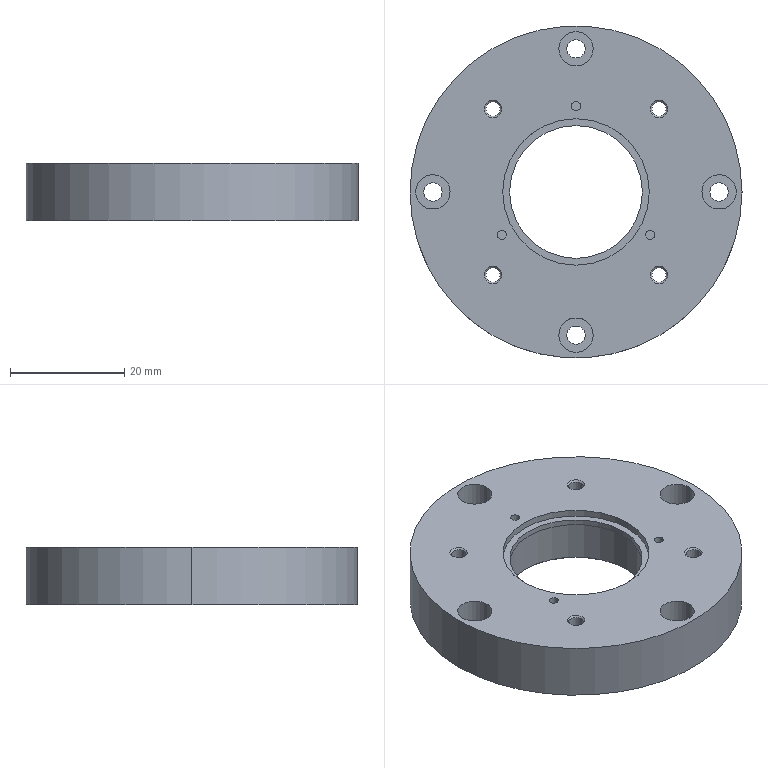Part | SolidWorks | features ICE 7, Cut 2, HoleWzd 2, MoveFace 2, Chamfer 1, Extrusion 1 | 1 solid | 59 faces | box 58 x 58 x 10 mm | volume 20570 mm3 | cylinder 38 | plane 11 | cone 10 | commonest cylinder face diameters 2.5 x8 3.2 x8 6 x8 1.6 x6 23.2 x2 25.1 x2